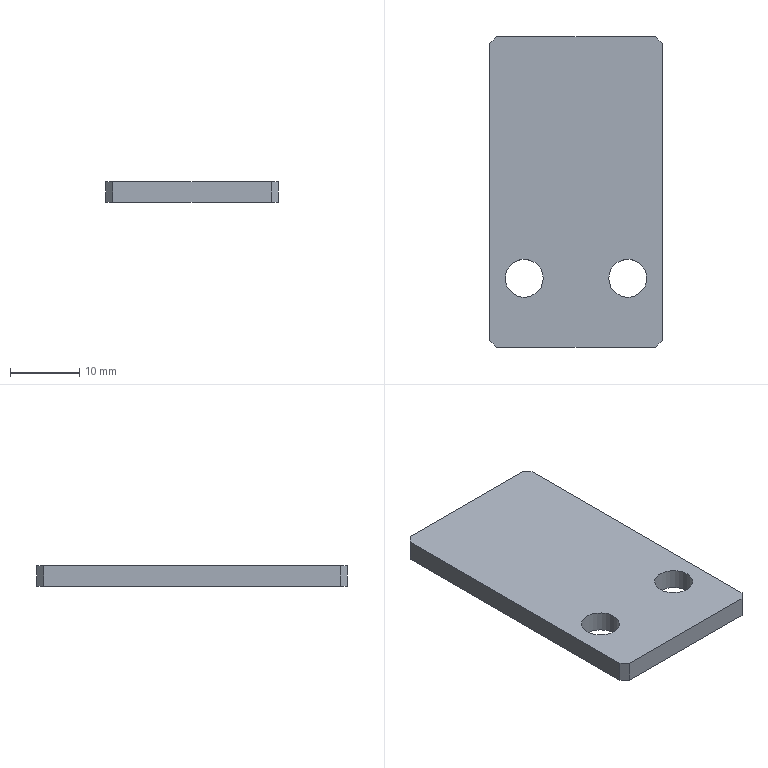Part | NX | 1 solid | 12 faces | box 25 x 45 x 3 mm | volume 3226 mm3 | plane 10 | cylinder 2 | commonest cylinder face diameters 5.5 x2
STEP:
#1=CARTESIAN_POINT('',(12.5,-21.5,0.));
#2=VERTEX_POINT('',#1);
#3=CARTESIAN_POINT('',(12.5,21.5,0.));
#4=VERTEX_POINT('',#3);
#5=CARTESIAN_POINT('',(12.5,-22.5,0.));
#6=DIRECTION('',(0.,1.,0.));
#7=VECTOR('',#6,1000.);
#8=LINE('',#5,#7);
#9=EDGE_CURVE('',#2,#4,#8,.T.);
#10=ORIENTED_EDGE('',*,*,#9,.F.);
#11=CARTESIAN_POINT('',(12.5,-21.5,-3.));
#12=VERTEX_POINT('',#11);
#13=CARTESIAN_POINT('',(12.5,-21.5,-3.));
#14=DIRECTION('',(0.,0.,-1.));
#15=VECTOR('',#14,1000.);
#16=LINE('',#13,#15);
#17=EDGE_CURVE('',#2,#12,#16,.T.);
#18=ORIENTED_EDGE('',*,*,#17,.T.);
#19=CARTESIAN_POINT('',(12.5,21.5,-3.));
#20=VERTEX_POINT('',#19);
#21=CARTESIAN_POINT('',(12.5,-22.5,-3.));
#22=DIRECTION('',(0.,1.,0.));
#23=VECTOR('',#22,1000.);
#24=LINE('',#21,#23);
#25=EDGE_CURVE('',#12,#20,#24,.T.);
#26=ORIENTED_EDGE('',*,*,#25,.T.);
#27=CARTESIAN_POINT('',(12.5,21.5,-3.));
#28=DIRECTION('',(0.,0.,1.));
#29=VECTOR('',#28,1000.);
#30=LINE('',#27,#29);
#31=EDGE_CURVE('',#20,#4,#30,.T.);
#32=ORIENTED_EDGE('',*,*,#31,.T.);
#33=EDGE_LOOP('',(#10,#18,#26,#32));
#34=FACE_BOUND('',#33,.T.);
#35=CARTESIAN_POINT('',(12.5,-22.5,-3.));
#36=DIRECTION('',(1.,0.,0.));
#37=DIRECTION('',(0.,0.,-1.));
#38=AXIS2_PLACEMENT_3D('',#35,#36,#37);
#39=PLANE('',#38);
#40=ADVANCED_FACE('',(#34),#39,.T.);
#41=CARTESIAN_POINT('',(-11.5,-22.5,-3.));
#42=VERTEX_POINT('',#41);
#43=CARTESIAN_POINT('',(11.5,-22.5,-3.));
#44=VERTEX_POINT('',#43);
#45=CARTESIAN_POINT('',(-12.5,-22.5,-3.));
#46=DIRECTION('',(1.,0.,0.));
#47=VECTOR('',#46,1000.);
#48=LINE('',#45,#47);
#49=EDGE_CURVE('',#42,#44,#48,.T.);
#50=ORIENTED_EDGE('',*,*,#49,.T.);
#51=CARTESIAN_POINT('',(11.5,-22.5,0.));
#52=VERTEX_POINT('',#51);
#53=CARTESIAN_POINT('',(11.5,-22.5,-3.));
#54=DIRECTION('',(0.,0.,1.));
#55=VECTOR('',#54,1000.);
#56=LINE('',#53,#55);
#57=EDGE_CURVE('',#44,#52,#56,.T.);
#58=ORIENTED_EDGE('',*,*,#57,.T.);
#59=CARTESIAN_POINT('',(-11.5,-22.5,0.));
#60=VERTEX_POINT('',#59);
#61=CARTESIAN_POINT('',(-12.5,-22.5,0.));
#62=DIRECTION('',(1.,0.,0.));
#63=VECTOR('',#62,1000.);
#64=LINE('',#61,#63);
#65=EDGE_CURVE('',#60,#52,#64,.T.);
#66=ORIENTED_EDGE('',*,*,#65,.F.);
#67=CARTESIAN_POINT('',(-11.5,-22.5,-3.));
#68=DIRECTION('',(0.,0.,-1.));
#69=VECTOR('',#68,1000.);
#70=LINE('',#67,#69);
#71=EDGE_CURVE('',#60,#42,#70,.T.);
#72=ORIENTED_EDGE('',*,*,#71,.T.);
#73=EDGE_LOOP('',(#50,#58,#66,#72));
#74=FACE_BOUND('',#73,.T.);
#75=CARTESIAN_POINT('',(-12.5,-22.5,-3.));
#76=DIRECTION('',(0.,-1.,0.));
#77=DIRECTION('',(0.,0.,-1.));
#78=AXIS2_PLACEMENT_3D('',#75,#76,#77);
#79=PLANE('',#78);
#80=ADVANCED_FACE('',(#74),#79,.T.);
#81=CARTESIAN_POINT('',(-12.5,21.5,-3.));
#82=VERTEX_POINT('',#81);
#83=CARTESIAN_POINT('',(-12.5,-21.5,-3.));
#84=VERTEX_POINT('',#83);
#85=CARTESIAN_POINT('',(-12.5,-22.5,-3.));
#86=DIRECTION('',(0.,-1.,0.));
#87=VECTOR('',#86,1000.);
#88=LINE('',#85,#87);
#89=EDGE_CURVE('',#82,#84,#88,.T.);
#90=ORIENTED_EDGE('',*,*,#89,.T.);
#91=CARTESIAN_POINT('',(-12.5,-21.5,0.));
#92=VERTEX_POINT('',#91);
#93=CARTESIAN_POINT('',(-12.5,-21.5,-3.));
#94=DIRECTION('',(0.,0.,1.));
#95=VECTOR('',#94,1000.);
#96=LINE('',#93,#95);
#97=EDGE_CURVE('',#84,#92,#96,.T.);
#98=ORIENTED_EDGE('',*,*,#97,.T.);
#99=CARTESIAN_POINT('',(-12.5,21.5,0.));
#100=VERTEX_POINT('',#99);
#101=CARTESIAN_POINT('',(-12.5,-22.5,0.));
#102=DIRECTION('',(0.,-1.,0.));
#103=VECTOR('',#102,1000.);
#104=LINE('',#101,#103);
#105=EDGE_CURVE('',#100,#92,#104,.T.);
#106=ORIENTED_EDGE('',*,*,#105,.F.);
#107=CARTESIAN_POINT('',(-12.5,21.5,-3.));
#108=DIRECTION('',(0.,0.,-1.));
#109=VECTOR('',#108,1000.);
#110=LINE('',#107,#109);
#111=EDGE_CURVE('',#100,#82,#110,.T.);
#112=ORIENTED_EDGE('',*,*,#111,.T.);
#113=EDGE_LOOP('',(#90,#98,#106,#112));
#114=FACE_BOUND('',#113,.T.);
#115=CARTESIAN_POINT('',(-12.5,-22.5,-3.));
#116=DIRECTION('',(-1.,0.,0.));
#117=DIRECTION('',(0.,0.,1.));
#118=AXIS2_PLACEMENT_3D('',#115,#116,#117);
#119=PLANE('',#118);
#120=ADVANCED_FACE('',(#114),#119,.T.);
#121=CARTESIAN_POINT('',(11.5,22.5,0.));
#122=VERTEX_POINT('',#121);
#123=CARTESIAN_POINT('',(-11.5,22.5,0.));
#124=VERTEX_POINT('',#123);
#125=CARTESIAN_POINT('',(-12.5,22.5,0.));
#126=DIRECTION('',(-1.,0.,0.));
#127=VECTOR('',#126,1000.);
#128=LINE('',#125,#127);
#129=EDGE_CURVE('',#122,#124,#128,.T.);
#130=ORIENTED_EDGE('',*,*,#129,.F.);
#131=CARTESIAN_POINT('',(11.5,22.5,-3.));
#132=VERTEX_POINT('',#131);
#133=CARTESIAN_POINT('',(11.5,22.5,-3.));
#134=DIRECTION('',(0.,0.,-1.));
#135=VECTOR('',#134,1000.);
#136=LINE('',#133,#135);
#137=EDGE_CURVE('',#122,#132,#136,.T.);
#138=ORIENTED_EDGE('',*,*,#137,.T.);
#139=CARTESIAN_POINT('',(-11.5,22.5,-3.));
#140=VERTEX_POINT('',#139);
#141=CARTESIAN_POINT('',(-12.5,22.5,-3.));
#142=DIRECTION('',(-1.,0.,0.));
#143=VECTOR('',#142,1000.);
#144=LINE('',#141,#143);
#145=EDGE_CURVE('',#132,#140,#144,.T.);
#146=ORIENTED_EDGE('',*,*,#145,.T.);
#147=CARTESIAN_POINT('',(-11.5,22.5,-3.));
#148=DIRECTION('',(0.,0.,1.));
#149=VECTOR('',#148,1000.);
#150=LINE('',#147,#149);
#151=EDGE_CURVE('',#140,#124,#150,.T.);
#152=ORIENTED_EDGE('',*,*,#151,.T.);
#153=EDGE_LOOP('',(#130,#138,#146,#152));
#154=FACE_BOUND('',#153,.T.);
#155=CARTESIAN_POINT('',(-12.5,22.5,-3.));
#156=DIRECTION('',(0.,1.,0.));
#157=DIRECTION('',(0.,0.,1.));
#158=AXIS2_PLACEMENT_3D('',#155,#156,#157);
#159=PLANE('',#158);
#160=ADVANCED_FACE('',(#154),#159,.T.);
#161=CARTESIAN_POINT('',(-4.75,-12.5,-3.));
#162=VERTEX_POINT('',#161);
#163=CARTESIAN_POINT('',(-7.5,-12.5,-3.));
#164=DIRECTION('',(0.,0.,1.));
#165=DIRECTION('',(1.,0.,0.));
#166=AXIS2_PLACEMENT_3D('',#163,#164,#165);
#167=CIRCLE('',#166,2.75);
#168=EDGE_CURVE('',#162,#162,#167,.T.);
#169=ORIENTED_EDGE('',*,*,#168,.T.);
#170=EDGE_LOOP('',(#169));
#171=FACE_BOUND('',#170,.T.);
#172=CARTESIAN_POINT('',(10.25,-12.5,-3.));
#173=VERTEX_POINT('',#172);
#174=CARTESIAN_POINT('',(7.5,-12.5,-3.));
#175=DIRECTION('',(0.,0.,1.));
#176=DIRECTION('',(1.,0.,0.));
#177=AXIS2_PLACEMENT_3D('',#174,#175,#176);
#178=CIRCLE('',#177,2.75);
#179=EDGE_CURVE('',#173,#173,#178,.T.);
#180=ORIENTED_EDGE('',*,*,#179,.T.);
#181=EDGE_LOOP('',(#180));
#182=FACE_BOUND('',#181,.T.);
#183=ORIENTED_EDGE('',*,*,#25,.F.);
#184=CARTESIAN_POINT('',(17.,-17.,-3.));
#185=DIRECTION('',(0.7071,0.7071,0.));
#186=VECTOR('',#185,1000.);
#187=LINE('',#184,#186);
#188=EDGE_CURVE('',#12,#44,#187,.F.);
#189=ORIENTED_EDGE('',*,*,#188,.T.);
#190=ORIENTED_EDGE('',*,*,#49,.F.);
#191=CARTESIAN_POINT('',(-17.,-17.,-3.));
#192=DIRECTION('',(0.7071,-0.7071,0.));
#193=VECTOR('',#192,1000.);
#194=LINE('',#191,#193);
#195=EDGE_CURVE('',#42,#84,#194,.F.);
#196=ORIENTED_EDGE('',*,*,#195,.T.);
#197=ORIENTED_EDGE('',*,*,#89,.F.);
#198=CARTESIAN_POINT('',(-17.,17.,-3.));
#199=DIRECTION('',(-0.7071,-0.7071,0.));
#200=VECTOR('',#199,1000.);
#201=LINE('',#198,#200);
#202=EDGE_CURVE('',#82,#140,#201,.F.);
#203=ORIENTED_EDGE('',*,*,#202,.T.);
#204=ORIENTED_EDGE('',*,*,#145,.F.);
#205=CARTESIAN_POINT('',(17.,17.,-3.));
#206=DIRECTION('',(-0.7071,0.7071,0.));
#207=VECTOR('',#206,1000.);
#208=LINE('',#205,#207);
#209=EDGE_CURVE('',#132,#20,#208,.F.);
#210=ORIENTED_EDGE('',*,*,#209,.T.);
#211=EDGE_LOOP('',(#183,#189,#190,#196,#197,#203,#204,#210));
#212=FACE_BOUND('',#211,.T.);
#213=CARTESIAN_POINT('',(0.,0.,-3.));
#214=DIRECTION('',(0.,0.,-1.));
#215=DIRECTION('',(-1.,0.,0.));
#216=AXIS2_PLACEMENT_3D('',#213,#214,#215);
#217=PLANE('',#216);
#218=ADVANCED_FACE('',(#171,#182,#212),#217,.T.);
#219=CARTESIAN_POINT('',(-4.75,-12.5,0.));
#220=VERTEX_POINT('',#219);
#221=CARTESIAN_POINT('',(-7.5,-12.5,0.));
#222=DIRECTION('',(0.,0.,1.));
#223=DIRECTION('',(1.,0.,0.));
#224=AXIS2_PLACEMENT_3D('',#221,#222,#223);
#225=CIRCLE('',#224,2.75);
#226=EDGE_CURVE('',#220,#220,#225,.T.);
#227=ORIENTED_EDGE('',*,*,#226,.F.);
#228=EDGE_LOOP('',(#227));
#229=FACE_BOUND('',#228,.T.);
#230=CARTESIAN_POINT('',(10.25,-12.5,0.));
#231=VERTEX_POINT('',#230);
#232=CARTESIAN_POINT('',(7.5,-12.5,0.));
#233=DIRECTION('',(0.,0.,1.));
#234=DIRECTION('',(1.,0.,0.));
#235=AXIS2_PLACEMENT_3D('',#232,#233,#234);
#236=CIRCLE('',#235,2.75);
#237=EDGE_CURVE('',#231,#231,#236,.T.);
#238=ORIENTED_EDGE('',*,*,#237,.F.);
#239=EDGE_LOOP('',(#238));
#240=FACE_BOUND('',#239,.T.);
#241=ORIENTED_EDGE('',*,*,#65,.T.);
#242=CARTESIAN_POINT('',(11.5,-22.5,0.));
#243=DIRECTION('',(-0.7071,-0.7071,0.));
#244=VECTOR('',#243,1000.);
#245=LINE('',#242,#244);
#246=EDGE_CURVE('',#52,#2,#245,.F.);
#247=ORIENTED_EDGE('',*,*,#246,.T.);
#248=ORIENTED_EDGE('',*,*,#9,.T.);
#249=CARTESIAN_POINT('',(12.5,21.5,0.));
#250=DIRECTION('',(0.7071,-0.7071,0.));
#251=VECTOR('',#250,1000.);
#252=LINE('',#249,#251);
#253=EDGE_CURVE('',#4,#122,#252,.F.);
#254=ORIENTED_EDGE('',*,*,#253,.T.);
#255=ORIENTED_EDGE('',*,*,#129,.T.);
#256=CARTESIAN_POINT('',(-11.5,22.5,0.));
#257=DIRECTION('',(0.7071,0.7071,0.));
#258=VECTOR('',#257,1000.);
#259=LINE('',#256,#258);
#260=EDGE_CURVE('',#124,#100,#259,.F.);
#261=ORIENTED_EDGE('',*,*,#260,.T.);
#262=ORIENTED_EDGE('',*,*,#105,.T.);
#263=CARTESIAN_POINT('',(-12.5,-21.5,0.));
#264=DIRECTION('',(-0.7071,0.7071,0.));
#265=VECTOR('',#264,1000.);
#266=LINE('',#263,#265);
#267=EDGE_CURVE('',#92,#60,#266,.F.);
#268=ORIENTED_EDGE('',*,*,#267,.T.);
#269=EDGE_LOOP('',(#241,#247,#248,#254,#255,#261,#262,#268));
#270=FACE_BOUND('',#269,.T.);
#271=CARTESIAN_POINT('',(0.,0.,0.));
#272=DIRECTION('',(0.,0.,-1.));
#273=DIRECTION('',(-1.,0.,0.));
#274=AXIS2_PLACEMENT_3D('',#271,#272,#273);
#275=PLANE('',#274);
#276=ADVANCED_FACE('',(#229,#240,#270),#275,.F.);
#277=ORIENTED_EDGE('',*,*,#179,.F.);
#278=EDGE_LOOP('',(#277));
#279=FACE_BOUND('',#278,.T.);
#280=ORIENTED_EDGE('',*,*,#237,.T.);
#281=EDGE_LOOP('',(#280));
#282=FACE_BOUND('',#281,.T.);
#283=CARTESIAN_POINT('',(7.5,-12.5,0.));
#284=DIRECTION('',(0.,0.,1.));
#285=DIRECTION('',(1.,0.,0.));
#286=AXIS2_PLACEMENT_3D('',#283,#284,#285);
#287=CYLINDRICAL_SURFACE('',#286,2.75);
#288=ADVANCED_FACE('',(#279,#282),#287,.F.);
#289=ORIENTED_EDGE('',*,*,#168,.F.);
#290=EDGE_LOOP('',(#289));
#291=FACE_BOUND('',#290,.T.);
#292=ORIENTED_EDGE('',*,*,#226,.T.);
#293=EDGE_LOOP('',(#292));
#294=FACE_BOUND('',#293,.T.);
#295=CARTESIAN_POINT('',(-7.5,-12.5,0.));
#296=DIRECTION('',(0.,0.,1.));
#297=DIRECTION('',(1.,0.,0.));
#298=AXIS2_PLACEMENT_3D('',#295,#296,#297);
#299=CYLINDRICAL_SURFACE('',#298,2.75);
#300=ADVANCED_FACE('',(#291,#294),#299,.F.);
#301=ORIENTED_EDGE('',*,*,#188,.F.);
#302=ORIENTED_EDGE('',*,*,#17,.F.);
#303=ORIENTED_EDGE('',*,*,#246,.F.);
#304=ORIENTED_EDGE('',*,*,#57,.F.);
#305=EDGE_LOOP('',(#301,#302,#303,#304));
#306=FACE_BOUND('',#305,.T.);
#307=CARTESIAN_POINT('',(11.5,-22.5,-3.));
#308=DIRECTION('',(-0.7071,0.7071,0.));
#309=DIRECTION('',(0.,0.,1.));
#310=AXIS2_PLACEMENT_3D('',#307,#308,#309);
#311=PLANE('',#310);
#312=ADVANCED_FACE('',(#306),#311,.F.);
#313=ORIENTED_EDGE('',*,*,#195,.F.);
#314=ORIENTED_EDGE('',*,*,#71,.F.);
#315=ORIENTED_EDGE('',*,*,#267,.F.);
#316=ORIENTED_EDGE('',*,*,#97,.F.);
#317=EDGE_LOOP('',(#313,#314,#315,#316));
#318=FACE_BOUND('',#317,.T.);
#319=CARTESIAN_POINT('',(-12.5,-21.5,-3.));
#320=DIRECTION('',(0.7071,0.7071,0.));
#321=DIRECTION('',(0.,0.,1.));
#322=AXIS2_PLACEMENT_3D('',#319,#320,#321);
#323=PLANE('',#322);
#324=ADVANCED_FACE('',(#318),#323,.F.);
#325=ORIENTED_EDGE('',*,*,#209,.F.);
#326=ORIENTED_EDGE('',*,*,#137,.F.);
#327=ORIENTED_EDGE('',*,*,#253,.F.);
#328=ORIENTED_EDGE('',*,*,#31,.F.);
#329=EDGE_LOOP('',(#325,#326,#327,#328));
#330=FACE_BOUND('',#329,.T.);
#331=CARTESIAN_POINT('',(12.5,21.5,-3.));
#332=DIRECTION('',(-0.7071,-0.7071,0.));
#333=DIRECTION('',(0.,0.,1.));
#334=AXIS2_PLACEMENT_3D('',#331,#332,#333);
#335=PLANE('',#334);
#336=ADVANCED_FACE('',(#330),#335,.F.);
#337=ORIENTED_EDGE('',*,*,#202,.F.);
#338=ORIENTED_EDGE('',*,*,#111,.F.);
#339=ORIENTED_EDGE('',*,*,#260,.F.);
#340=ORIENTED_EDGE('',*,*,#151,.F.);
#341=EDGE_LOOP('',(#337,#338,#339,#340));
#342=FACE_BOUND('',#341,.T.);
#343=CARTESIAN_POINT('',(-11.5,22.5,-3.));
#344=DIRECTION('',(0.7071,-0.7071,0.));
#345=DIRECTION('',(0.,0.,1.));
#346=AXIS2_PLACEMENT_3D('',#343,#344,#345);
#347=PLANE('',#346);
#348=ADVANCED_FACE('',(#342),#347,.F.);
#349=CLOSED_SHELL('',(#40,#80,#120,#160,#218,#276,#288,#300,#312,#324,#336,#348));
#350=MANIFOLD_SOLID_BREP('',#349);
#351=(LENGTH_UNIT()NAMED_UNIT(*)SI_UNIT(.MILLI.,.METRE.));
#352=UNCERTAINTY_MEASURE_WITH_UNIT(LENGTH_MEASURE(0.00001),#351,'','');
#353=(NAMED_UNIT(*)PLANE_ANGLE_UNIT()SI_UNIT($,.RADIAN.));
#354=(NAMED_UNIT(*)SI_UNIT($,.STERADIAN.)SOLID_ANGLE_UNIT());
#355=(GEOMETRIC_REPRESENTATION_CONTEXT(3)GLOBAL_UNCERTAINTY_ASSIGNED_CONTEXT((#352))GLOBAL_UNIT_ASSIGNED_CONTEXT((#351,#353,#354))REPRESENTATION_CONTEXT('',''));
#356=ADVANCED_BREP_SHAPE_REPRESENTATION('',(#350),#355);